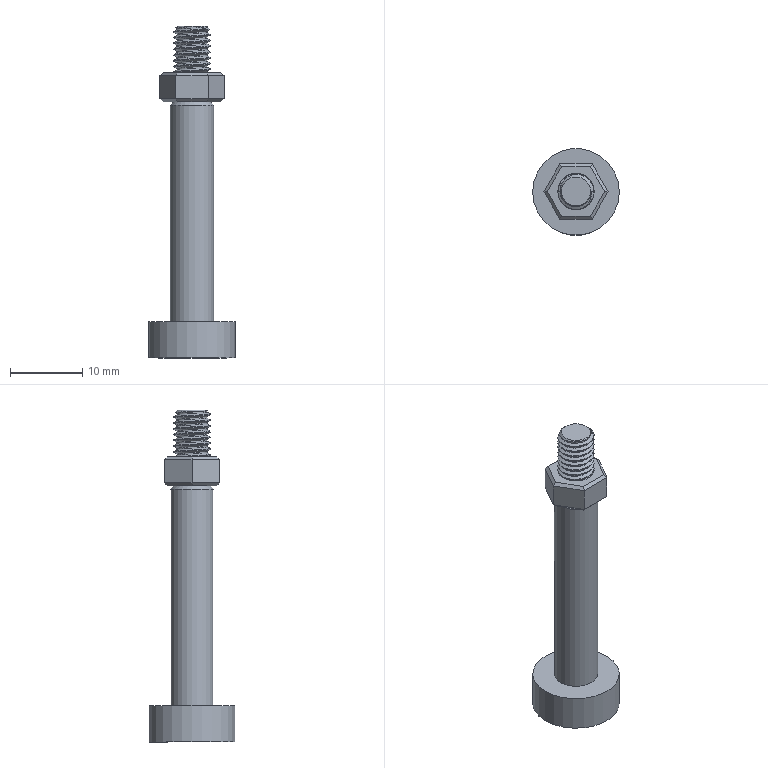Part | STEP file | 1 solid | 34 faces | box 12 x 12 x 46 mm | volume 1731 mm3 | plane 24 | cylinder 4 | cone 4 | spline 2 | commonest cylinder face diameters 4.2 x1 5 x1 6 x1 12 x1